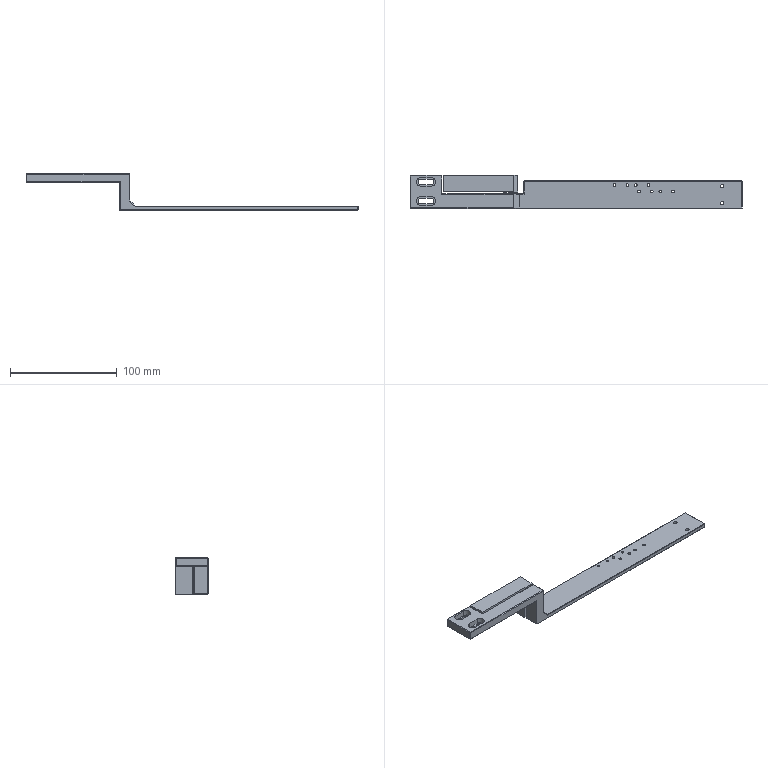NC program | NX | posted with a generic post | part box 311.5 x 31 x 34.5 mm
Whole program:
N10 G17 G21 G94 G90
(FLOOR_WALL_1_COPY_2 , TOOL : D10)
N12 T02 M6
N14 G54
N16 G17 G0 G90 X68.825 Y-8. B0. C0. S7000 M3
N18 G43 Z30. H2
N20 Z2.006
N22 G94 G1 Z-0.994 F1000.
N24 Y-5.
N26 X31.783 F2500.
N28 X35.15 Y-1.633
N30 Y9.633
N32 X31.783 Y13.
N34 X83.
N36 Y39.5
N38 X104.717
N40 X101.35 Y36.133
N42 Y28.867
N44 X104.717 Y25.5
N46 X104.571
N48 X102.5 Y23.429
N50 Y-5.
N52 X68.825
N54 Y2.
N56 X42.15
N58 Y6.
N60 X83.
N62 G3 X90. Y13. R7.
N64 G1 Y32.5
N66 X94.35
N68 Y28.867
N70 G3 X95.639 Y24.819 R7.
N72 X95.5 Y23.429 R7.
N74 G1 Y2.
N76 X68.825
N78 Y-8.
N80 Z2.006
N82 G0 Z30.
N84 Z1.012
N86 G1 Z-1.988 F1000.
N88 Y-5.
N90 X31.783 F2500.
N92 X35.15 Y-1.633
N94 Y9.633
N96 X31.783 Y13.
N98 X83.
N100 Y39.5
N102 X104.717
N104 X101.35 Y36.133
N106 Y28.867
N108 X104.717 Y25.5
N110 X104.571
N112 X102.5 Y23.429
N114 Y-5.
N116 X68.825
N118 Y2.
N120 X42.15
N122 Y6.
N124 X83.
N126 G3 X90. Y13. R7.
N128 G1 Y32.5
N130 X94.35
N132 Y28.867
N134 G3 X95.639 Y24.819 R7.
N136 X95.5 Y23.429 R7.
N138 G1 Y2.
N140 X68.825
N142 Y-8.
N144 Z1.012
N146 G0 Z30.
N148 Z0.018
N150 G1 Z-2.982 F1000.
N152 Y-5.
N154 X31.783 F2500.
N156 X35.15 Y-1.633
N158 Y9.633
N160 X31.783 Y13.
N162 X83.
N164 Y39.5
N166 X104.717
N168 X101.35 Y36.133
N170 Y28.867
N172 X104.717 Y25.5
N174 X104.571
N176 X102.5 Y23.429
N178 Y-5.
N180 X68.825
N182 Y2.
N184 X42.15
N186 Y6.
N188 X83.
N190 G3 X90. Y13. R7.
N192 G1 Y32.5
N194 X94.35
N196 Y28.867
N198 G3 X95.639 Y24.819 R7.
N200 X95.5 Y23.429 R7.
N202 G1 Y2.
N204 X68.825
N206 Y-8.
N208 Z0.018
N210 G0 Z30.
N212 Z-0.976
N214 G1 Z-3.976 F1000.
N216 Y-5.
N218 X31.783 F2500.
N220 X35.15 Y-1.633
N222 Y9.633
N224 X31.783 Y13.
N226 X83.
N228 Y39.5
N230 X104.717
N232 X101.35 Y36.133
N234 Y28.867
N236 X104.717 Y25.5
N238 X104.571
N240 X102.5 Y23.429
N242 Y-5.
N244 X68.825
N246 Y2.
N248 X42.15
N250 Y6.
N252 X83.
N254 G3 X90. Y13. R7.
N256 G1 Y32.5
N258 X94.35
N260 Y28.867
N262 G3 X95.639 Y24.819 R7.
N264 X95.5 Y23.429 R7.
N266 G1 Y2.
N268 X68.825
N270 Y-8.
N272 Z-0.976
N274 G0 Z30.
N276 Z-1.971
N278 G1 Z-4.971 F1000.
N280 Y-5.
N282 X31.783 F2500.
N284 X35.15 Y-1.633
N286 Y9.633
N288 X31.783 Y13.
N290 X83.
N292 Y39.5
N294 X104.717
N296 X101.35 Y36.133
N298 Y28.867
N300 X104.717 Y25.5
N302 X104.571
N304 X102.5 Y23.429
N306 Y-5.
N308 X68.825
N310 Y2.
N312 X42.15
N314 Y6.
N316 X83.
N318 G3 X90. Y13. R7.
N320 G1 Y32.5
N322 X94.35
N324 Y28.867
N326 G3 X95.639 Y24.819 R7.
N328 X95.5 Y23.429 R7.
N330 G1 Y2.
N332 X68.825
N334 Y-8.
N336 Z-1.971
N338 G0 Z30.
N340 Z-2.965
N342 G1 Z-5.965 F1000.
N344 Y-5.
N346 X31.783 F2500.
N348 X35.15 Y-1.633
N350 Y9.633
N352 X31.783 Y13.
N354 X83.
N356 Y39.5
N358 X104.717
N360 X101.35 Y36.133
N362 Y28.867
N364 X104.717 Y25.5
N366 X104.571
N368 X102.5 Y23.429
N370 Y-5.
N372 X68.825
N374 Y2.
N376 X42.15
N378 Y6.
N380 X83.
N382 G3 X90. Y13. R7.
N384 G1 Y32.5
N386 X94.35
N388 Y28.867
N390 G3 X95.639 Y24.819 R7.
N392 X95.5 Y23.429 R7.
N394 G1 Y2.
N396 X68.825
N398 Y-8.
N400 Z-2.965
N402 G0 Z30.
N404 Z-3.959
N406 G1 Z-6.959 F1000.
N408 Y-5.
N410 X31.783 F2500.
N412 X35.15 Y-1.633
N414 Y9.633
N416 X31.783 Y13.
N418 X83.
N420 Y39.5
N422 X104.717
N424 X101.35 Y36.133
N426 Y28.867
N428 X104.717 Y25.5
N430 X104.571
N432 X102.5 Y23.429
N434 Y-5.
N436 X68.825
N438 Y2.
N440 X42.15
N442 Y6.
N444 X83.
N446 G3 X90. Y13. R7.
N448 G1 Y32.5
N450 X94.35
N452 Y28.867
N454 G3 X95.639 Y24.819 R7.
N456 X95.5 Y23.429 R7.
N458 G1 Y2.
N460 X68.825
N462 Y-8.
N464 Z-3.959
N466 G0 Z30.
N468 Z-4.953
N470 G1 Z-7.953 F1000.
N472 Y-5.
N474 X31.783 F2500.
N476 X35.15 Y-1.633
N478 Y9.633
N480 X31.783 Y13.
N482 X83.
N484 Y39.5
N486 X104.717
N488 X101.35 Y36.133
N490 Y28.867
N492 X104.717 Y25.5
N494 X104.571
N496 X102.5 Y23.429
N498 Y-5.
N500 X68.825
N502 Y2.
N504 X42.15
N506 Y6.
N508 X83.
N510 G3 X90. Y13. R7.
N512 G1 Y32.5
N514 X94.35
N516 Y28.867
N518 G3 X95.639 Y24.819 R7.
N520 X95.5 Y23.429 R7.
N522 G1 Y2.
N524 X68.825
N526 Y-8.
N528 Z-4.953
N530 G0 Z30.
N532 Z-5.947
N534 G1 Z-8.947 F1000.
N536 Y-5.
N538 X31.783 F2500.
N540 X35.15 Y-1.633
N542 Y9.633
N544 X31.783 Y13.
N546 X83.
N548 Y39.5
N550 X104.717
N552 X101.35 Y36.133
N554 Y28.867
N556 X104.717 Y25.5
N558 X104.571
N560 X102.5 Y23.429
N562 Y-5.
N564 X68.825
N566 Y2.
N568 X42.15
N570 Y6.
N572 X83.
N574 G3 X90. Y13. R7.
N576 G1 Y32.5
N578 X94.35
N580 Y28.867
N582 G3 X95.639 Y24.819 R7.
N584 X95.5 Y23.429 R7.
N586 G1 Y2.
N588 X68.825
N590 Y-8.
N592 Z-5.947
N594 G0 Z30.
N596 Z-6.941
N598 G1 Z-9.941 F1000.
N600 Y-5.
N602 X31.783 F2500.
N604 X35.15 Y-1.633
N606 Y9.633
N608 X31.783 Y13.
N610 X83.
N612 Y39.5
N614 X104.717
N616 X101.35 Y36.133
N618 Y28.867
N620 X104.717 Y25.5
N622 X104.571
N624 X102.5 Y23.429
N626 Y-5.
N628 X68.825
N630 Y2.
N632 X42.15
N634 Y6.
N636 X83.
N638 G3 X90. Y13. R7.
N640 G1 Y32.5
N642 X94.35
N644 Y28.867
N646 G3 X95.639 Y24.819 R7.
N648 X95.5 Y23.429 R7.
N650 G1 Y2.
N652 X68.825
N654 Y-8.
N656 Z-6.941
N658 G0 Z30.
N660 Z-7.935
N662 G1 Z-10.935 F1000.
N664 Y-5.
N666 X31.783 F2500.
N668 X35.15 Y-1.633
N670 Y9.633
N672 X31.783 Y13.
N674 X83.
N676 Y39.5
N678 X104.717
N680 X101.35 Y36.133
N682 Y28.867
N684 X104.717 Y25.5
N686 X104.571
N688 X102.5 Y23.429
N690 Y-5.
N692 X68.825
N694 Y2.
N696 X42.15
N698 Y6.
N700 X83.
N702 G3 X90. Y13. R7.
N704 G1 Y32.5
N706 X94.35
N708 Y28.867
N710 G3 X95.639 Y24.819 R7.
N712 X95.5 Y23.429 R7.
N714 G1 Y2.
N716 X68.825
N718 Y-8.
N720 Z-7.935
N722 G0 Z30.
N724 Z-8.929
N726 G1 Z-11.929 F1000.
N728 Y-5.
N730 X31.783 F2500.
N732 X35.15 Y-1.633
N734 Y9.633
N736 X31.783 Y13.
N738 X83.
N740 Y39.5
N742 X104.717
N744 X101.35 Y36.133
N746 Y28.867
N748 X104.717 Y25.5
N750 X104.571
N752 X102.5 Y23.429
N754 Y-5.
N756 X68.825
N758 Y2.
N760 X42.15
N762 Y6.
N764 X83.
N766 G3 X90. Y13. R7.
N768 G1 Y32.5
N770 X94.35
N772 Y28.867
N774 G3 X95.639 Y24.819 R7.
N776 X95.5 Y23.429 R7.
N778 G1 Y2.
N780 X68.825
N782 Y-8.
N784 Z-8.929
N786 G0 Z30.
N788 Z-9.924
N790 G1 Z-12.924 F1000.
N792 Y-5.
N794 X31.783 F2500.
N796 X35.15 Y-1.633
N798 Y9.633
N800 X31.783 Y13.
N802 X83.
N804 Y39.5
N806 X104.717
N808 X101.35 Y36.133
N810 Y28.867
N812 X104.717 Y25.5
N814 X104.571
N816 X102.5 Y23.429
N818 Y-5.
N820 X68.825
N822 Y2.
N824 X42.15
N826 Y6.
N828 X83.
N830 G3 X90. Y13. R7.
N832 G1 Y32.5
N834 X94.35
N836 Y28.867
N838 G3 X95.639 Y24.819 R7.
N840 X95.5 Y23.429 R7.
N842 G1 Y2.
N844 X68.825
N846 Y-8.
N848 Z-9.924
N850 G0 Z30.
N852 Z-10.918
N854 G1 Z-13.918 F1000.
N856 Y-5.
N858 X31.783 F2500.
N860 X35.15 Y-1.633
N862 Y9.633
N864 X31.783 Y13.
N866 X83.
N868 Y39.5
N870 X104.717
N872 X101.35 Y36.133
N874 Y28.867
N876 X104.717 Y25.5
N878 X104.571
N880 X102.5 Y23.429
N882 Y-5.
N884 X68.825
N886 Y2.
N888 X42.15
N890 Y6.
N892 X83.
N894 G3 X90. Y13. R7.
N896 G1 Y32.5
N898 X94.35
N900 Y28.867
N902 G3 X95.639 Y24.819 R7.
N904 X95.5 Y23.429 R7.
N906 G1 Y2.
N908 X68.825
N910 Y-8.
N912 Z-10.918
N914 G0 Z30.
N916 Z-11.912
N918 G1 Z-14.912 F1000.
N920 Y-5.
N922 X31.783 F2500.
N924 X35.15 Y-1.633
N926 Y9.633
N928 X31.783 Y13.
N930 X83.
N932 Y39.5
N934 X104.717
N936 X101.35 Y36.133
N938 Y28.867
N940 X104.717 Y25.5
N942 X104.571
N944 X102.5 Y23.429
N946 Y-5.
N948 X68.825
N950 Y2.
N952 X42.15
N954 Y6.
N956 X83.
N958 G3 X90. Y13. R7.
N960 G1 Y32.5
N962 X94.35
N964 Y28.867
N966 G3 X95.639 Y24.819 R7.
N968 X95.5 Y23.429 R7.
N970 G1 Y2.
N972 X68.825
N974 Y-8.
N976 Z-11.912
N978 G0 Z30.
N980 Z-12.906
N982 G1 Z-15.906 F1000.
N984 Y-5.
N986 X31.783 F2500.
N988 X35.15 Y-1.633
N990 Y9.633
N992 X31.783 Y13.
N994 X83.
N996 Y39.5
N998 X104.717
N1000 X101.35 Y36.133
N1002 Y28.867
N1004 X104.717 Y25.5
N1006 X104.571
N1008 X102.5 Y23.429
N1010 Y-5.
N1012 X68.825
N1014 Y2.
N1016 X42.15
N1018 Y6.
N1020 X83.
N1022 G3 X90. Y13. R7.
N1024 G1 Y32.5
N1026 X94.35
N1028 Y28.867
N1030 G3 X95.639 Y24.819 R7.
N1032 X95.5 Y23.429 R7.
N1034 G1 Y2.
N1036 X68.825
N1038 Y-8.
N1040 Z-12.906
N1042 G0 Z30.
N1044 Z-13.9
N1046 G1 Z-16.9 F1000.
N1048 Y-5.
N1050 X31.783 F2500.
N1052 X35.15 Y-1.633
N1054 Y9.633
N1056 X31.783 Y13.
N1058 X83.
N1060 Y39.5
N1062 X104.717
N1064 X101.35 Y36.133
N1066 Y28.867
N1068 X104.717 Y25.5
N1070 X104.571
N1072 X102.5 Y23.429
N1074 Y-5.
N1076 X68.825
N1078 Y2.
N1080 X42.15
N1082 Y6.
N1084 X83.
N1086 G3 X90. Y13. R7.
N1088 G1 Y32.5
N1090 X94.35
N1092 Y28.867
N1094 G3 X95.639 Y24.819 R7.
N1096 X95.5 Y23.429 R7.
N1098 G1 Y2.
N1100 X68.825
N1102 Y-8.
N1104 Z-13.9
N1106 G0 Z30.
(FLOOR_WALL_1_COPY_COPY_COPY , TOOL : D10)
N1108 X101.3 Y36.935
N1110 Z-14.5
N1112 G1 Y39. Z-15.053 F1000.
N1114 Y36.578 Z-15.702
N1116 Y39. Z-16.351
N1118 Y36.578 Z-17.
N1120 Y39.
N1122 G2 X101.8 Y39.866 R1.
N1124 G1 X102.898 Y40.5
N1126 Z-15.5
N1128 G0 Z30.
N1130 X102.645 Y-5.854
N1132 Z-15.5
N1134 G1 Z-17.
N1136 X101.8 Y-5.366
N1138 G2 X101.3 Y-4.5 R1.
N1140 G1 Y28.422
N1142 Z-15.5
N1144 G0 Z-13.
N1146 G1 X98.198 Y40.5 F6000.
N1148 G0 Z-15.5
N1150 G1 Z-17. F1000.
N1152 X97.1 Y39.866
N1154 G3 X96.6 Y39. R1.
N1156 G1 Y-4.5
N1158 X91.9
N1160 Y39.
N1162 X87.2
N1164 Y-4.5
N1166 X82.5
N1168 Y12.5
N1170 X77.8
N1172 Y-4.5
N1174 X73.1
N1176 Y12.5
N1178 X68.4
N1180 Y-4.5
N1182 X63.7
N1184 Y12.5
N1186 X59.
N1188 Y-4.5
N1190 X54.3
N1192 Y12.5
N1194 X49.6
N1196 Y-4.5
N1198 X44.9
N1200 Y12.5
N1202 X40.2
N1204 Y-4.5
N1206 X35.5
N1208 Y12.5
N1210 G2 X36. Y13.366 R1.
N1212 G1 X37.098 Y14.
N1214 Z-15.5
N1216 G0 Z-13.
N1218 G1 X32.089 Y14.5 F6000.
N1220 G0 Z-15.5
N1222 G1 Z-17. F1000.
N1224 X31.812 Y13.466
N1226 G3 X32.071 Y12.5 R1.
N1228 G1 X35. Y9.571
N1230 Y-1.571
N1232 X32.071 Y-4.5
N1234 G3 X31.812 Y-5.466 R1.
N1236 G1 X32.089 Y-6.5
N1238 Z-15.5
N1240 G0 Z-13.
N1242 G1 X104.383 Y23.898 F6000.
N1244 G0 Z-15.5
N1246 G1 Z-17. F1000.
N1248 X104.688 Y25.034
N1250 G3 X104.429 Y26. R1.
N1252 G1 X101.5 Y28.929
N1254 Y36.071
N1256 X104.429 Y39.
N1258 G3 X104.688 Y39.966 R1.
N1260 G1 X104.411 Y41.
N1262 Z-15.5
N1264 G0 Z30.
N1266 M5
(ZLEVEL_PROFILE_COPY_1_COPY_COPY_COPY_COPY_COPY_1_COPY_1 , TOOL : D6A45)
N1268 T09 M6
N1270 G54
N1272 G17 G0 G90 X33.523 Y9.617 B0. C0. S7000 M3
N1274 G43 Z30. H9
N1276 Z-18.
N1278 G94 G1 X33.05 Y9.011 F1000.
N1280 G3 X32.967 Y8.417 R0.6
N1282 G1 X87.583
N1284 Y34.001
N1286 G2 X88.499 Y34.917 R0.925
N1288 G1 X103.529
N1290 G3 X103.444 Y35.511 R0.6
N1292 G1 X102.969 Y36.117
N1294 G0 Z30.
N1296 X102.404 Y28.117
N1298 Z-18.
N1300 G1 X103.457 Y29.488
N1302 G3 X103.536 Y30.083 R0.6
N1304 G1 X102.673
N1306 X97.917 Y25.327
N1308 Y0.499
N1310 G2 X97.001 Y-0.417 R0.916
N1312 G1 X32.97
N1314 G3 X33.049 Y-1.012 R0.6
N1316 G1 X33.514 Y-1.617
N1318 G0 Z30.
N1320 M5
N1322 M2